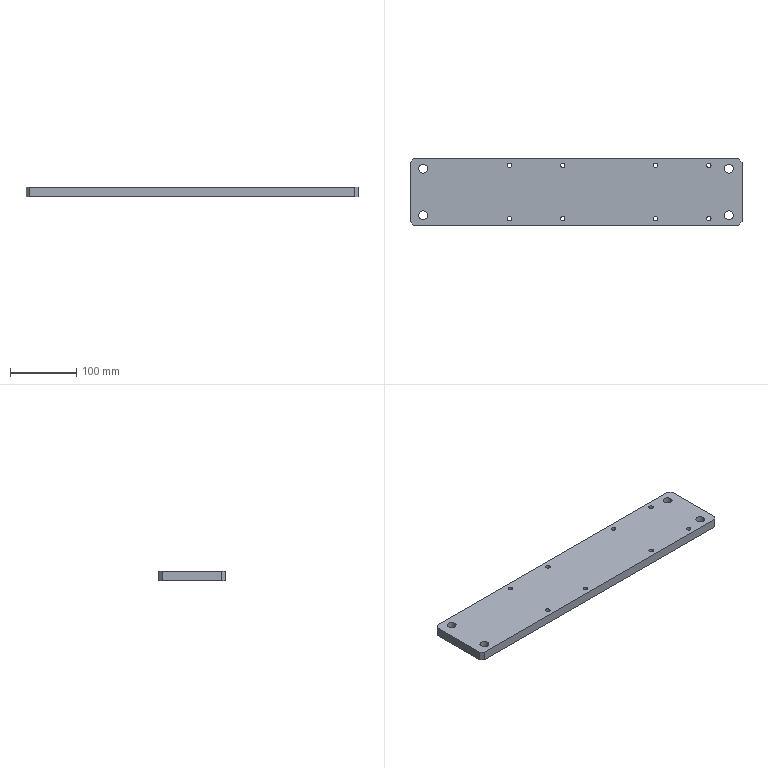Part | STEP file | Fixed Base Plate | 1 solid | 34 faces | box 500 x 100 x 14 mm | volume 687217 mm3 | cylinder 24 | plane 10 | commonest cylinder face diameters 6.8 x16 13.5 x8